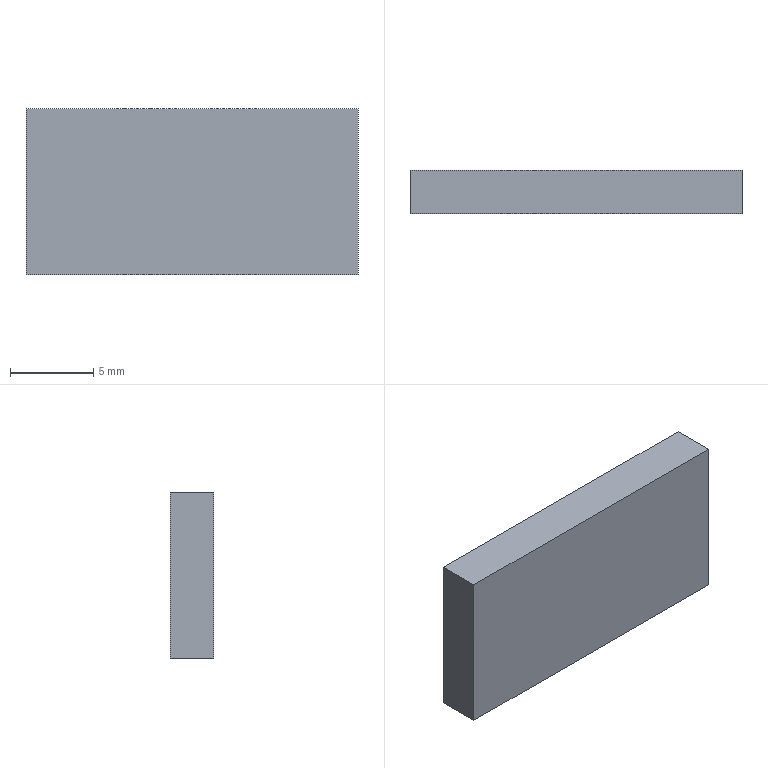Part | SolidWorks | features Extrusion 1 | 1 solid | 6 faces | box 20 x 2.6 x 10 mm | volume 520 mm3 | plane 6
STEP:
#1=CARTESIAN_POINT('',(10.,0.,5.));
#2=VERTEX_POINT('',#1);
#3=CARTESIAN_POINT('',(10.,0.,-5.));
#4=VERTEX_POINT('',#3);
#5=CARTESIAN_POINT('',(10.,0.,-5.));
#6=DIRECTION('',(0.,0.,-1.));
#7=VECTOR('',#6,1000.);
#8=LINE('',#5,#7);
#9=EDGE_CURVE('',#2,#4,#8,.T.);
#10=ORIENTED_EDGE('',*,*,#9,.T.);
#11=CARTESIAN_POINT('',(10.,2.6,-5.));
#12=VERTEX_POINT('',#11);
#13=CARTESIAN_POINT('',(10.,2.6,-5.));
#14=DIRECTION('',(0.,-1.,0.));
#15=VECTOR('',#14,1000.);
#16=LINE('',#13,#15);
#17=EDGE_CURVE('',#12,#4,#16,.T.);
#18=ORIENTED_EDGE('',*,*,#17,.F.);
#19=CARTESIAN_POINT('',(10.,2.6,5.));
#20=VERTEX_POINT('',#19);
#21=CARTESIAN_POINT('',(10.,2.6,-5.));
#22=DIRECTION('',(0.,0.,-1.));
#23=VECTOR('',#22,1000.);
#24=LINE('',#21,#23);
#25=EDGE_CURVE('',#20,#12,#24,.T.);
#26=ORIENTED_EDGE('',*,*,#25,.F.);
#27=CARTESIAN_POINT('',(10.,2.6,5.));
#28=DIRECTION('',(0.,-1.,0.));
#29=VECTOR('',#28,1000.);
#30=LINE('',#27,#29);
#31=EDGE_CURVE('',#20,#2,#30,.T.);
#32=ORIENTED_EDGE('',*,*,#31,.T.);
#33=EDGE_LOOP('',(#10,#18,#26,#32));
#34=FACE_OUTER_BOUND('',#33,.T.);
#35=CARTESIAN_POINT('',(10.,2.6,-5.));
#36=DIRECTION('',(-1.,0.,0.));
#37=DIRECTION('',(0.,0.,1.));
#38=AXIS2_PLACEMENT_3D('',#35,#36,#37);
#39=PLANE('',#38);
#40=ADVANCED_FACE('',(#34),#39,.F.);
#41=CARTESIAN_POINT('',(-10.,0.,-5.));
#42=VERTEX_POINT('',#41);
#43=CARTESIAN_POINT('',(-10.,0.,-5.));
#44=DIRECTION('',(-1.,0.,0.));
#45=VECTOR('',#44,1000.);
#46=LINE('',#43,#45);
#47=EDGE_CURVE('',#4,#42,#46,.T.);
#48=ORIENTED_EDGE('',*,*,#47,.T.);
#49=CARTESIAN_POINT('',(-10.,2.6,-5.));
#50=VERTEX_POINT('',#49);
#51=CARTESIAN_POINT('',(-10.,2.6,-5.));
#52=DIRECTION('',(0.,-1.,0.));
#53=VECTOR('',#52,1000.);
#54=LINE('',#51,#53);
#55=EDGE_CURVE('',#50,#42,#54,.T.);
#56=ORIENTED_EDGE('',*,*,#55,.F.);
#57=CARTESIAN_POINT('',(-10.,2.6,-5.));
#58=DIRECTION('',(-1.,0.,0.));
#59=VECTOR('',#58,1000.);
#60=LINE('',#57,#59);
#61=EDGE_CURVE('',#12,#50,#60,.T.);
#62=ORIENTED_EDGE('',*,*,#61,.F.);
#63=ORIENTED_EDGE('',*,*,#17,.T.);
#64=EDGE_LOOP('',(#48,#56,#62,#63));
#65=FACE_OUTER_BOUND('',#64,.T.);
#66=CARTESIAN_POINT('',(-10.,2.6,-5.));
#67=DIRECTION('',(0.,0.,1.));
#68=DIRECTION('',(1.,0.,0.));
#69=AXIS2_PLACEMENT_3D('',#66,#67,#68);
#70=PLANE('',#69);
#71=ADVANCED_FACE('',(#65),#70,.F.);
#72=CARTESIAN_POINT('',(-10.,0.,5.));
#73=VERTEX_POINT('',#72);
#74=CARTESIAN_POINT('',(-10.,0.,-5.));
#75=DIRECTION('',(0.,0.,1.));
#76=VECTOR('',#75,1000.);
#77=LINE('',#74,#76);
#78=EDGE_CURVE('',#42,#73,#77,.T.);
#79=ORIENTED_EDGE('',*,*,#78,.T.);
#80=CARTESIAN_POINT('',(-10.,2.6,5.));
#81=VERTEX_POINT('',#80);
#82=CARTESIAN_POINT('',(-10.,2.6,5.));
#83=DIRECTION('',(0.,-1.,0.));
#84=VECTOR('',#83,1000.);
#85=LINE('',#82,#84);
#86=EDGE_CURVE('',#81,#73,#85,.T.);
#87=ORIENTED_EDGE('',*,*,#86,.F.);
#88=CARTESIAN_POINT('',(-10.,2.6,-5.));
#89=DIRECTION('',(0.,0.,1.));
#90=VECTOR('',#89,1000.);
#91=LINE('',#88,#90);
#92=EDGE_CURVE('',#50,#81,#91,.T.);
#93=ORIENTED_EDGE('',*,*,#92,.F.);
#94=ORIENTED_EDGE('',*,*,#55,.T.);
#95=EDGE_LOOP('',(#79,#87,#93,#94));
#96=FACE_OUTER_BOUND('',#95,.T.);
#97=CARTESIAN_POINT('',(-10.,2.6,-5.));
#98=DIRECTION('',(1.,0.,0.));
#99=DIRECTION('',(0.,0.,-1.));
#100=AXIS2_PLACEMENT_3D('',#97,#98,#99);
#101=PLANE('',#100);
#102=ADVANCED_FACE('',(#96),#101,.F.);
#103=CARTESIAN_POINT('',(-10.,0.,5.));
#104=DIRECTION('',(1.,0.,0.));
#105=VECTOR('',#104,1000.);
#106=LINE('',#103,#105);
#107=EDGE_CURVE('',#73,#2,#106,.T.);
#108=ORIENTED_EDGE('',*,*,#107,.T.);
#109=ORIENTED_EDGE('',*,*,#31,.F.);
#110=CARTESIAN_POINT('',(-10.,2.6,5.));
#111=DIRECTION('',(1.,0.,0.));
#112=VECTOR('',#111,1000.);
#113=LINE('',#110,#112);
#114=EDGE_CURVE('',#81,#20,#113,.T.);
#115=ORIENTED_EDGE('',*,*,#114,.F.);
#116=ORIENTED_EDGE('',*,*,#86,.T.);
#117=EDGE_LOOP('',(#108,#109,#115,#116));
#118=FACE_OUTER_BOUND('',#117,.T.);
#119=CARTESIAN_POINT('',(-10.,2.6,5.));
#120=DIRECTION('',(0.,0.,-1.));
#121=DIRECTION('',(-1.,0.,0.));
#122=AXIS2_PLACEMENT_3D('',#119,#120,#121);
#123=PLANE('',#122);
#124=ADVANCED_FACE('',(#118),#123,.F.);
#125=ORIENTED_EDGE('',*,*,#25,.T.);
#126=ORIENTED_EDGE('',*,*,#61,.T.);
#127=ORIENTED_EDGE('',*,*,#92,.T.);
#128=ORIENTED_EDGE('',*,*,#114,.T.);
#129=EDGE_LOOP('',(#125,#126,#127,#128));
#130=FACE_OUTER_BOUND('',#129,.T.);
#131=CARTESIAN_POINT('',(0.,2.6,0.));
#132=DIRECTION('',(0.,1.,0.));
#133=DIRECTION('',(0.,0.,1.));
#134=AXIS2_PLACEMENT_3D('',#131,#132,#133);
#135=PLANE('',#134);
#136=ADVANCED_FACE('',(#130),#135,.T.);
#137=ORIENTED_EDGE('',*,*,#9,.F.);
#138=ORIENTED_EDGE('',*,*,#107,.F.);
#139=ORIENTED_EDGE('',*,*,#78,.F.);
#140=ORIENTED_EDGE('',*,*,#47,.F.);
#141=EDGE_LOOP('',(#137,#138,#139,#140));
#142=FACE_OUTER_BOUND('',#141,.T.);
#143=CARTESIAN_POINT('',(0.,0.,0.));
#144=DIRECTION('',(0.,1.,0.));
#145=DIRECTION('',(0.,0.,1.));
#146=AXIS2_PLACEMENT_3D('',#143,#144,#145);
#147=PLANE('',#146);
#148=ADVANCED_FACE('',(#142),#147,.F.);
#149=CLOSED_SHELL('',(#40,#71,#102,#124,#136,#148));
#150=MANIFOLD_SOLID_BREP('',#149);
#151=CARTESIAN_POINT('',(0.,0.,0.));
#152=DIRECTION('',(0.,0.,1.));
#153=DIRECTION('',(1.,0.,0.));
#154=AXIS2_PLACEMENT_3D('',#151,#152,#153);
#155=(LENGTH_UNIT()NAMED_UNIT(*)SI_UNIT(.MILLI.,.METRE.));
#156=UNCERTAINTY_MEASURE_WITH_UNIT(LENGTH_MEASURE(0.00001),#155,'','');
#157=(NAMED_UNIT(*)PLANE_ANGLE_UNIT()SI_UNIT($,.RADIAN.));
#158=(NAMED_UNIT(*)SI_UNIT($,.STERADIAN.)SOLID_ANGLE_UNIT());
#159=(GEOMETRIC_REPRESENTATION_CONTEXT(3)GLOBAL_UNCERTAINTY_ASSIGNED_CONTEXT((#156))GLOBAL_UNIT_ASSIGNED_CONTEXT((#155,#157,#158))REPRESENTATION_CONTEXT('',''));
#160=ADVANCED_BREP_SHAPE_REPRESENTATION('',(#150,#154),#159);